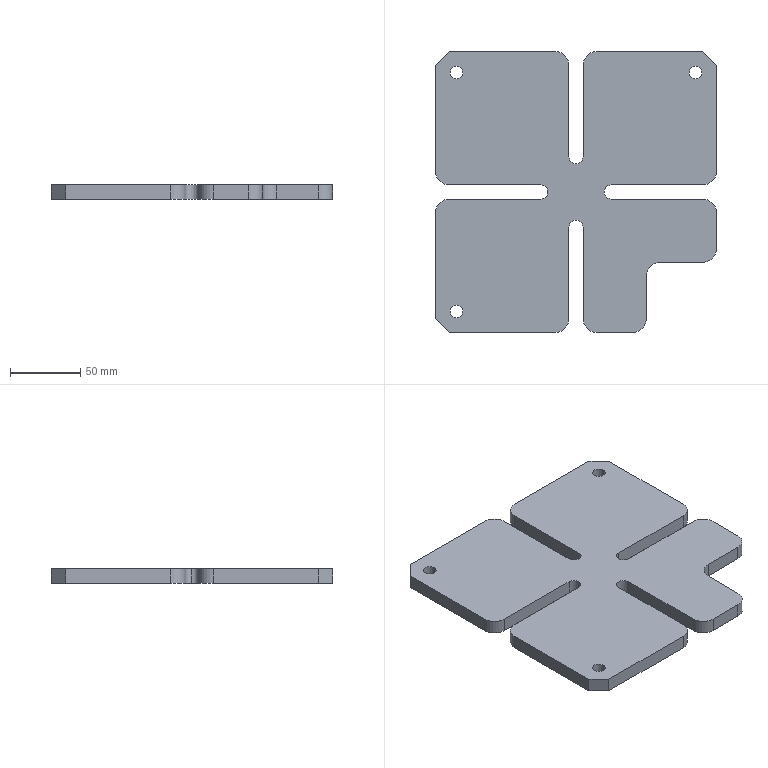Part | SolidWorks | features ICE 3, CirPattern 2, Fillet 2, Chamfer 1, DelFace 1, Extrusion 1, HoleWzd 1 | 1 solid | 45 faces | box 200 x 200 x 10 mm | volume 338089 mm3 | plane 23 | cylinder 22 | commonest cylinder face diameters 20 x11 9 x6 10 x5
STEP:
#1=CARTESIAN_POINT('',(-20.,0.,0.));
#2=VERTEX_POINT('',#1);
#3=CARTESIAN_POINT('',(-25.,5.,0.));
#4=VERTEX_POINT('',#3);
#5=CARTESIAN_POINT('',(-25.,0.,0.));
#6=DIRECTION('',(0.,0.,1.));
#7=DIRECTION('',(1.,0.,0.));
#8=AXIS2_PLACEMENT_3D('',#5,#6,#7);
#9=CIRCLE('',#8,5.);
#10=EDGE_CURVE('',#2,#4,#9,.T.);
#11=ORIENTED_EDGE('',*,*,#10,.F.);
#12=CARTESIAN_POINT('',(-20.,0.,10.));
#13=VERTEX_POINT('',#12);
#14=CARTESIAN_POINT('',(-20.,0.,-18.));
#15=DIRECTION('',(0.,0.,1.));
#16=VECTOR('',#15,1000.);
#17=LINE('',#14,#16);
#18=EDGE_CURVE('',#2,#13,#17,.T.);
#19=ORIENTED_EDGE('',*,*,#18,.T.);
#20=CARTESIAN_POINT('',(-25.,5.,10.));
#21=VERTEX_POINT('',#20);
#22=CARTESIAN_POINT('',(-25.,0.,10.));
#23=DIRECTION('',(0.,0.,1.));
#24=DIRECTION('',(1.,0.,0.));
#25=AXIS2_PLACEMENT_3D('',#22,#23,#24);
#26=CIRCLE('',#25,5.);
#27=EDGE_CURVE('',#13,#21,#26,.T.);
#28=ORIENTED_EDGE('',*,*,#27,.T.);
#29=CARTESIAN_POINT('',(-25.,5.,-18.));
#30=DIRECTION('',(0.,0.,1.));
#31=VECTOR('',#30,1000.);
#32=LINE('',#29,#31);
#33=EDGE_CURVE('',#4,#21,#32,.T.);
#34=ORIENTED_EDGE('',*,*,#33,.F.);
#35=EDGE_LOOP('',(#11,#19,#28,#34));
#36=FACE_OUTER_BOUND('',#35,.T.);
#37=CARTESIAN_POINT('',(-25.,0.,-18.));
#38=DIRECTION('',(0.,0.,1.));
#39=DIRECTION('',(1.,0.,0.));
#40=AXIS2_PLACEMENT_3D('',#37,#38,#39);
#41=CYLINDRICAL_SURFACE('',#40,5.);
#42=ADVANCED_FACE('',(#36),#41,.F.);
#43=CARTESIAN_POINT('',(80.5,85.,0.));
#44=VERTEX_POINT('',#43);
#45=CARTESIAN_POINT('',(89.5,85.,0.));
#46=VERTEX_POINT('',#45);
#47=CARTESIAN_POINT('',(85.,85.,0.));
#48=DIRECTION('',(0.,0.,1.));
#49=DIRECTION('',(1.,0.,0.));
#50=AXIS2_PLACEMENT_3D('',#47,#48,#49);
#51=CIRCLE('',#50,4.5);
#52=EDGE_CURVE('',#44,#46,#51,.T.);
#53=ORIENTED_EDGE('',*,*,#52,.F.);
#54=CARTESIAN_POINT('',(80.5,85.,10.));
#55=VERTEX_POINT('',#54);
#56=CARTESIAN_POINT('',(80.5,85.,10.));
#57=DIRECTION('',(0.,0.,1.));
#58=VECTOR('',#57,1000.);
#59=LINE('',#56,#58);
#60=EDGE_CURVE('',#44,#55,#59,.T.);
#61=ORIENTED_EDGE('',*,*,#60,.T.);
#62=CARTESIAN_POINT('',(89.5,85.,10.));
#63=VERTEX_POINT('',#62);
#64=CARTESIAN_POINT('',(85.,85.,10.));
#65=DIRECTION('',(0.,0.,1.));
#66=DIRECTION('',(1.,0.,0.));
#67=AXIS2_PLACEMENT_3D('',#64,#65,#66);
#68=CIRCLE('',#67,4.5);
#69=EDGE_CURVE('',#55,#63,#68,.T.);
#70=ORIENTED_EDGE('',*,*,#69,.T.);
#71=CARTESIAN_POINT('',(89.5,85.,10.));
#72=DIRECTION('',(0.,0.,1.));
#73=VECTOR('',#72,1000.);
#74=LINE('',#71,#73);
#75=EDGE_CURVE('',#46,#63,#74,.T.);
#76=ORIENTED_EDGE('',*,*,#75,.F.);
#77=EDGE_LOOP('',(#53,#61,#70,#76));
#78=FACE_OUTER_BOUND('',#77,.T.);
#79=CARTESIAN_POINT('',(85.,85.,10.));
#80=DIRECTION('',(0.,0.,1.));
#81=DIRECTION('',(1.,0.,0.));
#82=AXIS2_PLACEMENT_3D('',#79,#80,#81);
#83=CYLINDRICAL_SURFACE('',#82,4.5);
#84=ADVANCED_FACE('',(#78),#83,.F.);
#85=CARTESIAN_POINT('',(-89.5,85.,0.));
#86=VERTEX_POINT('',#85);
#87=CARTESIAN_POINT('',(-80.5,85.,0.));
#88=VERTEX_POINT('',#87);
#89=CARTESIAN_POINT('',(-85.,85.,0.));
#90=DIRECTION('',(0.,0.,1.));
#91=DIRECTION('',(1.,0.,0.));
#92=AXIS2_PLACEMENT_3D('',#89,#90,#91);
#93=CIRCLE('',#92,4.5);
#94=EDGE_CURVE('',#86,#88,#93,.T.);
#95=ORIENTED_EDGE('',*,*,#94,.F.);
#96=CARTESIAN_POINT('',(-89.5,85.,10.));
#97=VERTEX_POINT('',#96);
#98=CARTESIAN_POINT('',(-89.5,85.,10.));
#99=DIRECTION('',(0.,0.,1.));
#100=VECTOR('',#99,1000.);
#101=LINE('',#98,#100);
#102=EDGE_CURVE('',#86,#97,#101,.T.);
#103=ORIENTED_EDGE('',*,*,#102,.T.);
#104=CARTESIAN_POINT('',(-80.5,85.,10.));
#105=VERTEX_POINT('',#104);
#106=CARTESIAN_POINT('',(-85.,85.,10.));
#107=DIRECTION('',(0.,0.,1.));
#108=DIRECTION('',(1.,0.,0.));
#109=AXIS2_PLACEMENT_3D('',#106,#107,#108);
#110=CIRCLE('',#109,4.5);
#111=EDGE_CURVE('',#97,#105,#110,.T.);
#112=ORIENTED_EDGE('',*,*,#111,.T.);
#113=CARTESIAN_POINT('',(-80.5,85.,10.));
#114=DIRECTION('',(0.,0.,1.));
#115=VECTOR('',#114,1000.);
#116=LINE('',#113,#115);
#117=EDGE_CURVE('',#88,#105,#116,.T.);
#118=ORIENTED_EDGE('',*,*,#117,.F.);
#119=EDGE_LOOP('',(#95,#103,#112,#118));
#120=FACE_OUTER_BOUND('',#119,.T.);
#121=CARTESIAN_POINT('',(-85.,85.,10.));
#122=DIRECTION('',(0.,0.,1.));
#123=DIRECTION('',(1.,0.,0.));
#124=AXIS2_PLACEMENT_3D('',#121,#122,#123);
#125=CYLINDRICAL_SURFACE('',#124,4.5);
#126=ADVANCED_FACE('',(#120),#125,.F.);
#127=CARTESIAN_POINT('',(-89.5,-85.,0.));
#128=VERTEX_POINT('',#127);
#129=CARTESIAN_POINT('',(-80.5,-85.,0.));
#130=VERTEX_POINT('',#129);
#131=CARTESIAN_POINT('',(-85.,-85.,0.));
#132=DIRECTION('',(0.,0.,1.));
#133=DIRECTION('',(1.,0.,0.));
#134=AXIS2_PLACEMENT_3D('',#131,#132,#133);
#135=CIRCLE('',#134,4.5);
#136=EDGE_CURVE('',#128,#130,#135,.T.);
#137=ORIENTED_EDGE('',*,*,#136,.F.);
#138=CARTESIAN_POINT('',(-89.5,-85.,10.));
#139=VERTEX_POINT('',#138);
#140=CARTESIAN_POINT('',(-89.5,-85.,10.));
#141=DIRECTION('',(0.,0.,1.));
#142=VECTOR('',#141,1000.);
#143=LINE('',#140,#142);
#144=EDGE_CURVE('',#128,#139,#143,.T.);
#145=ORIENTED_EDGE('',*,*,#144,.T.);
#146=CARTESIAN_POINT('',(-80.5,-85.,10.));
#147=VERTEX_POINT('',#146);
#148=CARTESIAN_POINT('',(-85.,-85.,10.));
#149=DIRECTION('',(0.,0.,1.));
#150=DIRECTION('',(1.,0.,0.));
#151=AXIS2_PLACEMENT_3D('',#148,#149,#150);
#152=CIRCLE('',#151,4.5);
#153=EDGE_CURVE('',#139,#147,#152,.T.);
#154=ORIENTED_EDGE('',*,*,#153,.T.);
#155=CARTESIAN_POINT('',(-80.5,-85.,10.));
#156=DIRECTION('',(0.,0.,1.));
#157=VECTOR('',#156,1000.);
#158=LINE('',#155,#157);
#159=EDGE_CURVE('',#130,#147,#158,.T.);
#160=ORIENTED_EDGE('',*,*,#159,.F.);
#161=EDGE_LOOP('',(#137,#145,#154,#160));
#162=FACE_OUTER_BOUND('',#161,.T.);
#163=CARTESIAN_POINT('',(-85.,-85.,10.));
#164=DIRECTION('',(0.,0.,1.));
#165=DIRECTION('',(1.,0.,0.));
#166=AXIS2_PLACEMENT_3D('',#163,#164,#165);
#167=CYLINDRICAL_SURFACE('',#166,4.5);
#168=ADVANCED_FACE('',(#162),#167,.F.);
#169=CARTESIAN_POINT('',(100.,15.,10.));
#170=VERTEX_POINT('',#169);
#171=CARTESIAN_POINT('',(100.,90.,10.));
#172=VERTEX_POINT('',#171);
#173=CARTESIAN_POINT('',(100.,100.,10.));
#174=DIRECTION('',(0.,1.,0.));
#175=VECTOR('',#174,1000.);
#176=LINE('',#173,#175);
#177=EDGE_CURVE('',#170,#172,#176,.T.);
#178=ORIENTED_EDGE('',*,*,#177,.F.);
#179=CARTESIAN_POINT('',(100.,15.,0.));
#180=VERTEX_POINT('',#179);
#181=CARTESIAN_POINT('',(100.,15.,10.));
#182=DIRECTION('',(0.,0.,-1.));
#183=VECTOR('',#182,1000.);
#184=LINE('',#181,#183);
#185=EDGE_CURVE('',#170,#180,#184,.T.);
#186=ORIENTED_EDGE('',*,*,#185,.T.);
#187=CARTESIAN_POINT('',(100.,90.,0.));
#188=VERTEX_POINT('',#187);
#189=CARTESIAN_POINT('',(100.,100.,0.));
#190=DIRECTION('',(0.,1.,0.));
#191=VECTOR('',#190,1000.);
#192=LINE('',#189,#191);
#193=EDGE_CURVE('',#180,#188,#192,.T.);
#194=ORIENTED_EDGE('',*,*,#193,.T.);
#195=CARTESIAN_POINT('',(100.,90.,10.));
#196=DIRECTION('',(0.,0.,1.));
#197=VECTOR('',#196,1000.);
#198=LINE('',#195,#197);
#199=EDGE_CURVE('',#188,#172,#198,.T.);
#200=ORIENTED_EDGE('',*,*,#199,.T.);
#201=EDGE_LOOP('',(#178,#186,#194,#200));
#202=FACE_OUTER_BOUND('',#201,.T.);
#203=CARTESIAN_POINT('',(100.,100.,10.));
#204=DIRECTION('',(-1.,0.,0.));
#205=DIRECTION('',(0.,-1.,0.));
#206=AXIS2_PLACEMENT_3D('',#203,#204,#205);
#207=PLANE('',#206);
#208=ADVANCED_FACE('',(#202),#207,.F.);
#209=CARTESIAN_POINT('',(-15.,100.,10.));
#210=VERTEX_POINT('',#209);
#211=CARTESIAN_POINT('',(-90.,100.,10.));
#212=VERTEX_POINT('',#211);
#213=CARTESIAN_POINT('',(-100.,100.,10.));
#214=DIRECTION('',(-1.,0.,0.));
#215=VECTOR('',#214,1000.);
#216=LINE('',#213,#215);
#217=EDGE_CURVE('',#210,#212,#216,.T.);
#218=ORIENTED_EDGE('',*,*,#217,.F.);
#219=CARTESIAN_POINT('',(-15.,100.,0.));
#220=VERTEX_POINT('',#219);
#221=CARTESIAN_POINT('',(-15.,100.,10.));
#222=DIRECTION('',(0.,0.,-1.));
#223=VECTOR('',#222,1000.);
#224=LINE('',#221,#223);
#225=EDGE_CURVE('',#210,#220,#224,.T.);
#226=ORIENTED_EDGE('',*,*,#225,.T.);
#227=CARTESIAN_POINT('',(-90.,100.,0.));
#228=VERTEX_POINT('',#227);
#229=CARTESIAN_POINT('',(-100.,100.,0.));
#230=DIRECTION('',(-1.,0.,0.));
#231=VECTOR('',#230,1000.);
#232=LINE('',#229,#231);
#233=EDGE_CURVE('',#220,#228,#232,.T.);
#234=ORIENTED_EDGE('',*,*,#233,.T.);
#235=CARTESIAN_POINT('',(-90.,100.,10.));
#236=DIRECTION('',(0.,0.,1.));
#237=VECTOR('',#236,1000.);
#238=LINE('',#235,#237);
#239=EDGE_CURVE('',#228,#212,#238,.T.);
#240=ORIENTED_EDGE('',*,*,#239,.T.);
#241=EDGE_LOOP('',(#218,#226,#234,#240));
#242=FACE_OUTER_BOUND('',#241,.T.);
#243=CARTESIAN_POINT('',(-100.,100.,10.));
#244=DIRECTION('',(0.,-1.,0.));
#245=DIRECTION('',(0.,0.,-1.));
#246=AXIS2_PLACEMENT_3D('',#243,#244,#245);
#247=PLANE('',#246);
#248=ADVANCED_FACE('',(#242),#247,.F.);
#249=CARTESIAN_POINT('',(15.,-100.,0.));
#250=VERTEX_POINT('',#249);
#251=CARTESIAN_POINT('',(40.,-100.,0.));
#252=VERTEX_POINT('',#251);
#253=CARTESIAN_POINT('',(-100.,-100.,0.));
#254=DIRECTION('',(1.,0.,0.));
#255=VECTOR('',#254,1000.);
#256=LINE('',#253,#255);
#257=EDGE_CURVE('',#250,#252,#256,.T.);
#258=ORIENTED_EDGE('',*,*,#257,.T.);
#259=CARTESIAN_POINT('',(40.,-100.,10.));
#260=VERTEX_POINT('',#259);
#261=CARTESIAN_POINT('',(40.,-100.,10.));
#262=DIRECTION('',(0.,0.,1.));
#263=VECTOR('',#262,1000.);
#264=LINE('',#261,#263);
#265=EDGE_CURVE('',#252,#260,#264,.T.);
#266=ORIENTED_EDGE('',*,*,#265,.T.);
#267=CARTESIAN_POINT('',(15.,-100.,10.));
#268=VERTEX_POINT('',#267);
#269=CARTESIAN_POINT('',(-100.,-100.,10.));
#270=DIRECTION('',(1.,0.,0.));
#271=VECTOR('',#270,1000.);
#272=LINE('',#269,#271);
#273=EDGE_CURVE('',#268,#260,#272,.T.);
#274=ORIENTED_EDGE('',*,*,#273,.F.);
#275=CARTESIAN_POINT('',(15.,-100.,10.));
#276=DIRECTION('',(0.,0.,-1.));
#277=VECTOR('',#276,1000.);
#278=LINE('',#275,#277);
#279=EDGE_CURVE('',#268,#250,#278,.T.);
#280=ORIENTED_EDGE('',*,*,#279,.T.);
#281=EDGE_LOOP('',(#258,#266,#274,#280));
#282=FACE_OUTER_BOUND('',#281,.T.);
#283=CARTESIAN_POINT('',(-100.,-100.,10.));
#284=DIRECTION('',(0.,1.,0.));
#285=DIRECTION('',(0.,0.,1.));
#286=AXIS2_PLACEMENT_3D('',#283,#284,#285);
#287=PLANE('',#286);
#288=ADVANCED_FACE('',(#282),#287,.F.);
#289=CARTESIAN_POINT('',(-100.,-15.,10.));
#290=VERTEX_POINT('',#289);
#291=CARTESIAN_POINT('',(-100.,-90.,10.));
#292=VERTEX_POINT('',#291);
#293=CARTESIAN_POINT('',(-100.,100.,10.));
#294=DIRECTION('',(0.,-1.,0.));
#295=VECTOR('',#294,1000.);
#296=LINE('',#293,#295);
#297=EDGE_CURVE('',#290,#292,#296,.T.);
#298=ORIENTED_EDGE('',*,*,#297,.F.);
#299=CARTESIAN_POINT('',(-100.,-15.,0.));
#300=VERTEX_POINT('',#299);
#301=CARTESIAN_POINT('',(-100.,-15.,10.));
#302=DIRECTION('',(0.,0.,-1.));
#303=VECTOR('',#302,1000.);
#304=LINE('',#301,#303);
#305=EDGE_CURVE('',#290,#300,#304,.T.);
#306=ORIENTED_EDGE('',*,*,#305,.T.);
#307=CARTESIAN_POINT('',(-100.,-90.,0.));
#308=VERTEX_POINT('',#307);
#309=CARTESIAN_POINT('',(-100.,100.,0.));
#310=DIRECTION('',(0.,-1.,0.));
#311=VECTOR('',#310,1000.);
#312=LINE('',#309,#311);
#313=EDGE_CURVE('',#300,#308,#312,.T.);
#314=ORIENTED_EDGE('',*,*,#313,.T.);
#315=CARTESIAN_POINT('',(-100.,-90.,10.));
#316=DIRECTION('',(0.,0.,1.));
#317=VECTOR('',#316,1000.);
#318=LINE('',#315,#317);
#319=EDGE_CURVE('',#308,#292,#318,.T.);
#320=ORIENTED_EDGE('',*,*,#319,.T.);
#321=EDGE_LOOP('',(#298,#306,#314,#320));
#322=FACE_OUTER_BOUND('',#321,.T.);
#323=CARTESIAN_POINT('',(-100.,100.,10.));
#324=DIRECTION('',(1.,0.,0.));
#325=DIRECTION('',(0.,1.,0.));
#326=AXIS2_PLACEMENT_3D('',#323,#324,#325);
#327=PLANE('',#326);
#328=ADVANCED_FACE('',(#322),#327,.F.);
#329=CARTESIAN_POINT('',(100.,-40.,10.));
#330=VERTEX_POINT('',#329);
#331=CARTESIAN_POINT('',(100.,-15.,10.));
#332=VERTEX_POINT('',#331);
#333=CARTESIAN_POINT('',(100.,100.,10.));
#334=DIRECTION('',(0.,1.,0.));
#335=VECTOR('',#334,1000.);
#336=LINE('',#333,#335);
#337=EDGE_CURVE('',#330,#332,#336,.T.);
#338=ORIENTED_EDGE('',*,*,#337,.F.);
#339=CARTESIAN_POINT('',(100.,-40.,0.));
#340=VERTEX_POINT('',#339);
#341=CARTESIAN_POINT('',(100.,-40.,10.));
#342=DIRECTION('',(0.,0.,-1.));
#343=VECTOR('',#342,1000.);
#344=LINE('',#341,#343);
#345=EDGE_CURVE('',#330,#340,#344,.T.);
#346=ORIENTED_EDGE('',*,*,#345,.T.);
#347=CARTESIAN_POINT('',(100.,-15.,0.));
#348=VERTEX_POINT('',#347);
#349=CARTESIAN_POINT('',(100.,100.,0.));
#350=DIRECTION('',(0.,1.,0.));
#351=VECTOR('',#350,1000.);
#352=LINE('',#349,#351);
#353=EDGE_CURVE('',#340,#348,#352,.T.);
#354=ORIENTED_EDGE('',*,*,#353,.T.);
#355=CARTESIAN_POINT('',(100.,-15.,10.));
#356=DIRECTION('',(0.,0.,1.));
#357=VECTOR('',#356,1000.);
#358=LINE('',#355,#357);
#359=EDGE_CURVE('',#348,#332,#358,.T.);
#360=ORIENTED_EDGE('',*,*,#359,.T.);
#361=EDGE_LOOP('',(#338,#346,#354,#360));
#362=FACE_OUTER_BOUND('',#361,.T.);
#363=CARTESIAN_POINT('',(100.,100.,10.));
#364=DIRECTION('',(-1.,0.,0.));
#365=DIRECTION('',(0.,-1.,0.));
#366=AXIS2_PLACEMENT_3D('',#363,#364,#365);
#367=PLANE('',#366);
#368=ADVANCED_FACE('',(#362),#367,.F.);
#369=CARTESIAN_POINT('',(90.,100.,0.));
#370=VERTEX_POINT('',#369);
#371=CARTESIAN_POINT('',(15.,100.,0.));
#372=VERTEX_POINT('',#371);
#373=CARTESIAN_POINT('',(-100.,100.,0.));
#374=DIRECTION('',(-1.,0.,0.));
#375=VECTOR('',#374,1000.);
#376=LINE('',#373,#375);
#377=EDGE_CURVE('',#370,#372,#376,.T.);
#378=ORIENTED_EDGE('',*,*,#377,.T.);
#379=CARTESIAN_POINT('',(15.,100.,10.));
#380=VERTEX_POINT('',#379);
#381=CARTESIAN_POINT('',(15.,100.,10.));
#382=DIRECTION('',(0.,0.,1.));
#383=VECTOR('',#382,1000.);
#384=LINE('',#381,#383);
#385=EDGE_CURVE('',#372,#380,#384,.T.);
#386=ORIENTED_EDGE('',*,*,#385,.T.);
#387=CARTESIAN_POINT('',(90.,100.,10.));
#388=VERTEX_POINT('',#387);
#389=CARTESIAN_POINT('',(-100.,100.,10.));
#390=DIRECTION('',(-1.,0.,0.));
#391=VECTOR('',#390,1000.);
#392=LINE('',#389,#391);
#393=EDGE_CURVE('',#388,#380,#392,.T.);
#394=ORIENTED_EDGE('',*,*,#393,.F.);
#395=CARTESIAN_POINT('',(90.,100.,10.));
#396=DIRECTION('',(0.,0.,-1.));
#397=VECTOR('',#396,1000.);
#398=LINE('',#395,#397);
#399=EDGE_CURVE('',#388,#370,#398,.T.);
#400=ORIENTED_EDGE('',*,*,#399,.T.);
#401=EDGE_LOOP('',(#378,#386,#394,#400));
#402=FACE_OUTER_BOUND('',#401,.T.);
#403=CARTESIAN_POINT('',(-100.,100.,10.));
#404=DIRECTION('',(0.,-1.,0.));
#405=DIRECTION('',(0.,0.,-1.));
#406=AXIS2_PLACEMENT_3D('',#403,#404,#405);
#407=PLANE('',#406);
#408=ADVANCED_FACE('',(#402),#407,.F.);
#409=CARTESIAN_POINT('',(-100.,90.,0.));
#410=VERTEX_POINT('',#409);
#411=CARTESIAN_POINT('',(-100.,15.,0.));
#412=VERTEX_POINT('',#411);
#413=CARTESIAN_POINT('',(-100.,100.,0.));
#414=DIRECTION('',(0.,-1.,0.));
#415=VECTOR('',#414,1000.);
#416=LINE('',#413,#415);
#417=EDGE_CURVE('',#410,#412,#416,.T.);
#418=ORIENTED_EDGE('',*,*,#417,.T.);
#419=CARTESIAN_POINT('',(-100.,15.,10.));
#420=VERTEX_POINT('',#419);
#421=CARTESIAN_POINT('',(-100.,15.,10.));
#422=DIRECTION('',(0.,0.,1.));
#423=VECTOR('',#422,1000.);
#424=LINE('',#421,#423);
#425=EDGE_CURVE('',#412,#420,#424,.T.);
#426=ORIENTED_EDGE('',*,*,#425,.T.);
#427=CARTESIAN_POINT('',(-100.,90.,10.));
#428=VERTEX_POINT('',#427);
#429=CARTESIAN_POINT('',(-100.,100.,10.));
#430=DIRECTION('',(0.,-1.,0.));
#431=VECTOR('',#430,1000.);
#432=LINE('',#429,#431);
#433=EDGE_CURVE('',#428,#420,#432,.T.);
#434=ORIENTED_EDGE('',*,*,#433,.F.);
#435=CARTESIAN_POINT('',(-100.,90.,10.));
#436=DIRECTION('',(0.,0.,-1.));
#437=VECTOR('',#436,1000.);
#438=LINE('',#435,#437);
#439=EDGE_CURVE('',#428,#410,#438,.T.);
#440=ORIENTED_EDGE('',*,*,#439,.T.);
#441=EDGE_LOOP('',(#418,#426,#434,#440));
#442=FACE_OUTER_BOUND('',#441,.T.);
#443=CARTESIAN_POINT('',(-100.,100.,10.));
#444=DIRECTION('',(1.,0.,0.));
#445=DIRECTION('',(0.,1.,0.));
#446=AXIS2_PLACEMENT_3D('',#443,#444,#445);
#447=PLANE('',#446);
#448=ADVANCED_FACE('',(#442),#447,.F.);
#449=CARTESIAN_POINT('',(-90.,-100.,0.));
#450=VERTEX_POINT('',#449);
#451=CARTESIAN_POINT('',(-15.,-100.,0.));
#452=VERTEX_POINT('',#451);
#453=CARTESIAN_POINT('',(-100.,-100.,0.));
#454=DIRECTION('',(1.,0.,0.));
#455=VECTOR('',#454,1000.);
#456=LINE('',#453,#455);
#457=EDGE_CURVE('',#450,#452,#456,.T.);
#458=ORIENTED_EDGE('',*,*,#457,.T.);
#459=CARTESIAN_POINT('',(-15.,-100.,10.));
#460=VERTEX_POINT('',#459);
#461=CARTESIAN_POINT('',(-15.,-100.,10.));
#462=DIRECTION('',(0.,0.,1.));
#463=VECTOR('',#462,1000.);
#464=LINE('',#461,#463);
#465=EDGE_CURVE('',#452,#460,#464,.T.);
#466=ORIENTED_EDGE('',*,*,#465,.T.);
#467=CARTESIAN_POINT('',(-90.,-100.,10.));
#468=VERTEX_POINT('',#467);
#469=CARTESIAN_POINT('',(-100.,-100.,10.));
#470=DIRECTION('',(1.,0.,0.));
#471=VECTOR('',#470,1000.);
#472=LINE('',#469,#471);
#473=EDGE_CURVE('',#468,#460,#472,.T.);
#474=ORIENTED_EDGE('',*,*,#473,.F.);
#475=CARTESIAN_POINT('',(-90.,-100.,10.));
#476=DIRECTION('',(0.,0.,-1.));
#477=VECTOR('',#476,1000.);
#478=LINE('',#475,#477);
#479=EDGE_CURVE('',#468,#450,#478,.T.);
#480=ORIENTED_EDGE('',*,*,#479,.T.);
#481=EDGE_LOOP('',(#458,#466,#474,#480));
#482=FACE_OUTER_BOUND('',#481,.T.);
#483=CARTESIAN_POINT('',(-100.,-100.,10.));
#484=DIRECTION('',(0.,1.,0.));
#485=DIRECTION('',(0.,0.,1.));
#486=AXIS2_PLACEMENT_3D('',#483,#484,#485);
#487=PLANE('',#486);
#488=ADVANCED_FACE('',(#482),#487,.F.);
#489=ORIENTED_EDGE('',*,*,#273,.T.);
#490=CARTESIAN_POINT('',(50.,-90.,10.));
#491=VERTEX_POINT('',#490);
#492=CARTESIAN_POINT('',(40.,-90.,10.));
#493=DIRECTION('',(0.,0.,1.));
#494=DIRECTION('',(1.,0.,0.));
#495=AXIS2_PLACEMENT_3D('',#492,#493,#494);
#496=CIRCLE('',#495,10.);
#497=EDGE_CURVE('',#260,#491,#496,.T.);
#498=ORIENTED_EDGE('',*,*,#497,.T.);
#499=CARTESIAN_POINT('',(50.,-60.,10.));
#500=VERTEX_POINT('',#499);
#501=CARTESIAN_POINT('',(50.,-50.,10.));
#502=DIRECTION('',(0.,-1.,0.));
#503=VECTOR('',#502,1000.);
#504=LINE('',#501,#503);
#505=EDGE_CURVE('',#500,#491,#504,.T.);
#506=ORIENTED_EDGE('',*,*,#505,.F.);
#507=CARTESIAN_POINT('',(60.,-50.,10.));
#508=VERTEX_POINT('',#507);
#509=CARTESIAN_POINT('',(60.,-60.,10.));
#510=DIRECTION('',(0.,0.,-1.));
#511=DIRECTION('',(1.,0.,0.));
#512=AXIS2_PLACEMENT_3D('',#509,#510,#511);
#513=CIRCLE('',#512,10.);
#514=EDGE_CURVE('',#500,#508,#513,.T.);
#515=ORIENTED_EDGE('',*,*,#514,.T.);
#516=CARTESIAN_POINT('',(90.,-50.,10.));
#517=VERTEX_POINT('',#516);
#518=CARTESIAN_POINT('',(50.,-50.,10.));
#519=DIRECTION('',(-1.,0.,0.));
#520=VECTOR('',#519,1000.);
#521=LINE('',#518,#520);
#522=EDGE_CURVE('',#517,#508,#521,.T.);
#523=ORIENTED_EDGE('',*,*,#522,.F.);
#524=CARTESIAN_POINT('',(90.,-40.,10.));
#525=DIRECTION('',(0.,0.,1.));
#526=DIRECTION('',(1.,0.,0.));
#527=AXIS2_PLACEMENT_3D('',#524,#525,#526);
#528=CIRCLE('',#527,10.);
#529=EDGE_CURVE('',#517,#330,#528,.T.);
#530=ORIENTED_EDGE('',*,*,#529,.T.);
#531=ORIENTED_EDGE('',*,*,#337,.T.);
#532=CARTESIAN_POINT('',(90.,-5.,10.));
#533=VERTEX_POINT('',#532);
#534=CARTESIAN_POINT('',(90.,-15.,10.));
#535=DIRECTION('',(0.,0.,1.));
#536=DIRECTION('',(1.,0.,0.));
#537=AXIS2_PLACEMENT_3D('',#534,#535,#536);
#538=CIRCLE('',#537,10.);
#539=EDGE_CURVE('',#332,#533,#538,.T.);
#540=ORIENTED_EDGE('',*,*,#539,.T.);
#541=CARTESIAN_POINT('',(25.,-5.,10.));
#542=VERTEX_POINT('',#541);
#543=CARTESIAN_POINT('',(25.,-5.,10.));
#544=DIRECTION('',(1.,0.,0.));
#545=VECTOR('',#544,1000.);
#546=LINE('',#543,#545);
#547=EDGE_CURVE('',#542,#533,#546,.T.);
#548=ORIENTED_EDGE('',*,*,#547,.F.);
#549=CARTESIAN_POINT('',(25.,5.,10.));
#550=VERTEX_POINT('',#549);
#551=CARTESIAN_POINT('',(25.,0.,10.));
#552=DIRECTION('',(0.,0.,1.));
#553=DIRECTION('',(-1.,0.,0.));
#554=AXIS2_PLACEMENT_3D('',#551,#552,#553);
#555=CIRCLE('',#554,5.);
#556=EDGE_CURVE('',#550,#542,#555,.T.);
#557=ORIENTED_EDGE('',*,*,#556,.F.);
#558=CARTESIAN_POINT('',(90.,5.,10.));
#559=VERTEX_POINT('',#558);
#560=CARTESIAN_POINT('',(25.,5.,10.));
#561=DIRECTION('',(-1.,0.,0.));
#562=VECTOR('',#561,1000.);
#563=LINE('',#560,#562);
#564=EDGE_CURVE('',#559,#550,#563,.T.);
#565=ORIENTED_EDGE('',*,*,#564,.F.);
#566=CARTESIAN_POINT('',(90.,15.,10.));
#567=DIRECTION('',(0.,0.,1.));
#568=DIRECTION('',(1.,0.,0.));
#569=AXIS2_PLACEMENT_3D('',#566,#567,#568);
#570=CIRCLE('',#569,10.);
#571=EDGE_CURVE('',#559,#170,#570,.T.);
#572=ORIENTED_EDGE('',*,*,#571,.T.);
#573=ORIENTED_EDGE('',*,*,#177,.T.);
#574=CARTESIAN_POINT('',(95.,95.,10.));
#575=DIRECTION('',(-0.7071,0.7071,0.));
#576=VECTOR('',#575,1000.);
#577=LINE('',#574,#576);
#578=EDGE_CURVE('',#172,#388,#577,.T.);
#579=ORIENTED_EDGE('',*,*,#578,.T.);
#580=ORIENTED_EDGE('',*,*,#393,.T.);
#581=CARTESIAN_POINT('',(5.,90.,10.));
#582=VERTEX_POINT('',#581);
#583=CARTESIAN_POINT('',(15.,90.,10.));
#584=DIRECTION('',(0.,0.,1.));
#585=DIRECTION('',(1.,0.,0.));
#586=AXIS2_PLACEMENT_3D('',#583,#584,#585);
#587=CIRCLE('',#586,10.);
#588=EDGE_CURVE('',#380,#582,#587,.T.);
#589=ORIENTED_EDGE('',*,*,#588,.T.);
#590=CARTESIAN_POINT('',(5.,25.,10.));
#591=VERTEX_POINT('',#590);
#592=CARTESIAN_POINT('',(5.,25.,10.));
#593=DIRECTION('',(0.,1.,0.));
#594=VECTOR('',#593,1000.);
#595=LINE('',#592,#594);
#596=EDGE_CURVE('',#591,#582,#595,.T.);
#597=ORIENTED_EDGE('',*,*,#596,.F.);
#598=CARTESIAN_POINT('',(-5.,25.,10.));
#599=VERTEX_POINT('',#598);
#600=CARTESIAN_POINT('',(0.,25.,10.));
#601=DIRECTION('',(0.,0.,1.));
#602=DIRECTION('',(0.,-1.,0.));
#603=AXIS2_PLACEMENT_3D('',#600,#601,#602);
#604=CIRCLE('',#603,5.);
#605=EDGE_CURVE('',#599,#591,#604,.T.);
#606=ORIENTED_EDGE('',*,*,#605,.F.);
#607=CARTESIAN_POINT('',(-5.,90.,10.));
#608=VERTEX_POINT('',#607);
#609=CARTESIAN_POINT('',(-5.,25.,10.));
#610=DIRECTION('',(0.,-1.,0.));
#611=VECTOR('',#610,1000.);
#612=LINE('',#609,#611);
#613=EDGE_CURVE('',#608,#599,#612,.T.);
#614=ORIENTED_EDGE('',*,*,#613,.F.);
#615=CARTESIAN_POINT('',(-15.,90.,10.));
#616=DIRECTION('',(0.,0.,1.));
#617=DIRECTION('',(1.,0.,0.));
#618=AXIS2_PLACEMENT_3D('',#615,#616,#617);
#619=CIRCLE('',#618,10.);
#620=EDGE_CURVE('',#608,#210,#619,.T.);
#621=ORIENTED_EDGE('',*,*,#620,.T.);
#622=ORIENTED_EDGE('',*,*,#217,.T.);
#623=CARTESIAN_POINT('',(-95.,95.,10.));
#624=DIRECTION('',(-0.7071,-0.7071,0.));
#625=VECTOR('',#624,1000.);
#626=LINE('',#623,#625);
#627=EDGE_CURVE('',#212,#428,#626,.T.);
#628=ORIENTED_EDGE('',*,*,#627,.T.);
#629=ORIENTED_EDGE('',*,*,#433,.T.);
#630=CARTESIAN_POINT('',(-90.,5.,10.));
#631=VERTEX_POINT('',#630);
#632=CARTESIAN_POINT('',(-90.,15.,10.));
#633=DIRECTION('',(0.,0.,1.));
#634=DIRECTION('',(1.,0.,0.));
#635=AXIS2_PLACEMENT_3D('',#632,#633,#634);
#636=CIRCLE('',#635,10.);
#637=EDGE_CURVE('',#420,#631,#636,.T.);
#638=ORIENTED_EDGE('',*,*,#637,.T.);
#639=CARTESIAN_POINT('',(-25.,5.,10.));
#640=DIRECTION('',(-1.,0.,0.));
#641=VECTOR('',#640,1000.);
#642=LINE('',#639,#641);
#643=EDGE_CURVE('',#21,#631,#642,.T.);
#644=ORIENTED_EDGE('',*,*,#643,.F.);
#645=ORIENTED_EDGE('',*,*,#27,.F.);
#646=CARTESIAN_POINT('',(-25.,-5.,10.));
#647=VERTEX_POINT('',#646);
#648=CARTESIAN_POINT('',(-25.,0.,10.));
#649=DIRECTION('',(0.,0.,1.));
#650=DIRECTION('',(1.,0.,0.));
#651=AXIS2_PLACEMENT_3D('',#648,#649,#650);
#652=CIRCLE('',#651,5.);
#653=EDGE_CURVE('',#647,#13,#652,.T.);
#654=ORIENTED_EDGE('',*,*,#653,.F.);
#655=CARTESIAN_POINT('',(-90.,-5.,10.));
#656=VERTEX_POINT('',#655);
#657=CARTESIAN_POINT('',(-25.,-5.,10.));
#658=DIRECTION('',(1.,0.,0.));
#659=VECTOR('',#658,1000.);
#660=LINE('',#657,#659);
#661=EDGE_CURVE('',#656,#647,#660,.T.);
#662=ORIENTED_EDGE('',*,*,#661,.F.);
#663=CARTESIAN_POINT('',(-90.,-15.,10.));
#664=DIRECTION('',(0.,0.,1.));
#665=DIRECTION('',(1.,0.,0.));
#666=AXIS2_PLACEMENT_3D('',#663,#664,#665);
#667=CIRCLE('',#666,10.);
#668=EDGE_CURVE('',#656,#290,#667,.T.);
#669=ORIENTED_EDGE('',*,*,#668,.T.);
#670=ORIENTED_EDGE('',*,*,#297,.T.);
#671=CARTESIAN_POINT('',(-95.,-95.,10.));
#672=DIRECTION('',(0.7071,-0.7071,0.));
#673=VECTOR('',#672,1000.);
#674=LINE('',#671,#673);
#675=EDGE_CURVE('',#292,#468,#674,.T.);
#676=ORIENTED_EDGE('',*,*,#675,.T.);
#677=ORIENTED_EDGE('',*,*,#473,.T.);
#678=CARTESIAN_POINT('',(-5.,-90.,10.));
#679=VERTEX_POINT('',#678);
#680=CARTESIAN_POINT('',(-15.,-90.,10.));
#681=DIRECTION('',(0.,0.,1.));
#682=DIRECTION('',(1.,0.,0.));
#683=AXIS2_PLACEMENT_3D('',#680,#681,#682);
#684=CIRCLE('',#683,10.);
#685=EDGE_CURVE('',#460,#679,#684,.T.);
#686=ORIENTED_EDGE('',*,*,#685,.T.);
#687=CARTESIAN_POINT('',(-5.,-25.,10.));
#688=VERTEX_POINT('',#687);
#689=CARTESIAN_POINT('',(-5.,-25.,10.));
#690=DIRECTION('',(0.,-1.,0.));
#691=VECTOR('',#690,1000.);
#692=LINE('',#689,#691);
#693=EDGE_CURVE('',#688,#679,#692,.T.);
#694=ORIENTED_EDGE('',*,*,#693,.F.);
#695=CARTESIAN_POINT('',(5.,-25.,10.));
#696=VERTEX_POINT('',#695);
#697=CARTESIAN_POINT('',(0.,-25.,10.));
#698=DIRECTION('',(0.,0.,1.));
#699=DIRECTION('',(0.,1.,0.));
#700=AXIS2_PLACEMENT_3D('',#697,#698,#699);
#701=CIRCLE('',#700,5.);
#702=EDGE_CURVE('',#696,#688,#701,.T.);
#703=ORIENTED_EDGE('',*,*,#702,.F.);
#704=CARTESIAN_POINT('',(5.,-90.,10.));
#705=VERTEX_POINT('',#704);
#706=CARTESIAN_POINT('',(5.,-25.,10.));
#707=DIRECTION('',(0.,1.,0.));
#708=VECTOR('',#707,1000.);
#709=LINE('',#706,#708);
#710=EDGE_CURVE('',#705,#696,#709,.T.);
#711=ORIENTED_EDGE('',*,*,#710,.F.);
#712=CARTESIAN_POINT('',(15.,-90.,10.));
#713=DIRECTION('',(0.,0.,1.));
#714=DIRECTION('',(1.,0.,0.));
#715=AXIS2_PLACEMENT_3D('',#712,#713,#714);
#716=CIRCLE('',#715,10.);
#717=EDGE_CURVE('',#705,#268,#716,.T.);
#718=ORIENTED_EDGE('',*,*,#717,.T.);
#719=EDGE_LOOP('',(#489,#498,#506,#515,#523,#530,#531,#540,#548,#557,#565,#572,#573,#579,#580,#589,#597,#606,#614,#621,#622,#628,#629,#638,#644,#645,#654,#662,#669,#670,#676,#677,#686,#694,#703,#711,#718));
#720=FACE_OUTER_BOUND('',#719,.T.);
#721=CARTESIAN_POINT('',(85.,85.,10.));
#722=DIRECTION('',(0.,0.,1.));
#723=DIRECTION('',(1.,0.,0.));
#724=AXIS2_PLACEMENT_3D('',#721,#722,#723);
#725=CIRCLE('',#724,4.5);
#726=EDGE_CURVE('',#63,#55,#725,.T.);
#727=ORIENTED_EDGE('',*,*,#726,.F.);
#728=ORIENTED_EDGE('',*,*,#69,.F.);
#729=EDGE_LOOP('',(#727,#728));
#730=FACE_BOUND('',#729,.T.);
#731=CARTESIAN_POINT('',(-85.,85.,10.));
#732=DIRECTION('',(0.,0.,1.));
#733=DIRECTION('',(1.,0.,0.));
#734=AXIS2_PLACEMENT_3D('',#731,#732,#733);
#735=CIRCLE('',#734,4.5);
#736=EDGE_CURVE('',#105,#97,#735,.T.);
#737=ORIENTED_EDGE('',*,*,#736,.F.);
#738=ORIENTED_EDGE('',*,*,#111,.F.);
#739=EDGE_LOOP('',(#737,#738));
#740=FACE_BOUND('',#739,.T.);
#741=CARTESIAN_POINT('',(-85.,-85.,10.));
#742=DIRECTION('',(0.,0.,1.));
#743=DIRECTION('',(1.,0.,0.));
#744=AXIS2_PLACEMENT_3D('',#741,#742,#743);
#745=CIRCLE('',#744,4.5);
#746=EDGE_CURVE('',#147,#139,#745,.T.);
#747=ORIENTED_EDGE('',*,*,#746,.F.);
#748=ORIENTED_EDGE('',*,*,#153,.F.);
#749=EDGE_LOOP('',(#747,#748));
#750=FACE_BOUND('',#749,.T.);
#751=CARTESIAN_POINT('',(0.,0.,10.));
#752=DIRECTION('',(0.,0.,1.));
#753=DIRECTION('',(1.,0.,0.));
#754=AXIS2_PLACEMENT_3D('',#751,#752,#753);
#755=PLANE('',#754);
#756=ADVANCED_FACE('',(#720,#730,#740,#750),#755,.T.);
#757=CARTESIAN_POINT('',(85.,85.,0.));
#758=DIRECTION('',(0.,0.,1.));
#759=DIRECTION('',(1.,0.,0.));
#760=AXIS2_PLACEMENT_3D('',#757,#758,#759);
#761=CIRCLE('',#760,4.5);
#762=EDGE_CURVE('',#46,#44,#761,.T.);
#763=ORIENTED_EDGE('',*,*,#762,.T.);
#764=ORIENTED_EDGE('',*,*,#52,.T.);
#765=EDGE_LOOP('',(#763,#764));
#766=FACE_BOUND('',#765,.T.);
#767=CARTESIAN_POINT('',(-85.,85.,0.));
#768=DIRECTION('',(0.,0.,1.));
#769=DIRECTION('',(1.,0.,0.));
#770=AXIS2_PLACEMENT_3D('',#767,#768,#769);
#771=CIRCLE('',#770,4.5);
#772=EDGE_CURVE('',#88,#86,#771,.T.);
#773=ORIENTED_EDGE('',*,*,#772,.T.);
#774=ORIENTED_EDGE('',*,*,#94,.T.);
#775=EDGE_LOOP('',(#773,#774));
#776=FACE_BOUND('',#775,.T.);
#777=CARTESIAN_POINT('',(-85.,-85.,0.));
#778=DIRECTION('',(0.,0.,1.));
#779=DIRECTION('',(1.,0.,0.));
#780=AXIS2_PLACEMENT_3D('',#777,#778,#779);
#781=CIRCLE('',#780,4.5);
#782=EDGE_CURVE('',#130,#128,#781,.T.);
#783=ORIENTED_EDGE('',*,*,#782,.T.);
#784=ORIENTED_EDGE('',*,*,#136,.T.);
#785=EDGE_LOOP('',(#783,#784));
#786=FACE_BOUND('',#785,.T.);
#787=CARTESIAN_POINT('',(50.,-60.,0.));
#788=VERTEX_POINT('',#787);
#789=CARTESIAN_POINT('',(50.,-90.,0.));
#790=VERTEX_POINT('',#789);
#791=CARTESIAN_POINT('',(50.,-50.,0.));
#792=DIRECTION('',(0.,-1.,0.));
#793=VECTOR('',#792,1000.);
#794=LINE('',#791,#793);
#795=EDGE_CURVE('',#788,#790,#794,.T.);
#796=ORIENTED_EDGE('',*,*,#795,.T.);
#797=CARTESIAN_POINT('',(40.,-90.,0.));
#798=DIRECTION('',(0.,0.,-1.));
#799=DIRECTION('',(1.,0.,0.));
#800=AXIS2_PLACEMENT_3D('',#797,#798,#799);
#801=CIRCLE('',#800,10.);
#802=EDGE_CURVE('',#790,#252,#801,.T.);
#803=ORIENTED_EDGE('',*,*,#802,.T.);
#804=ORIENTED_EDGE('',*,*,#257,.F.);
#805=CARTESIAN_POINT('',(5.,-90.,0.));
#806=VERTEX_POINT('',#805);
#807=CARTESIAN_POINT('',(15.,-90.,0.));
#808=DIRECTION('',(0.,0.,-1.));
#809=DIRECTION('',(1.,0.,0.));
#810=AXIS2_PLACEMENT_3D('',#807,#808,#809);
#811=CIRCLE('',#810,10.);
#812=EDGE_CURVE('',#250,#806,#811,.T.);
#813=ORIENTED_EDGE('',*,*,#812,.T.);
#814=CARTESIAN_POINT('',(5.,-25.,0.));
#815=VERTEX_POINT('',#814);
#816=CARTESIAN_POINT('',(5.,0.,0.));
#817=DIRECTION('',(0.,1.,0.));
#818=VECTOR('',#817,1000.);
#819=LINE('',#816,#818);
#820=EDGE_CURVE('',#806,#815,#819,.T.);
#821=ORIENTED_EDGE('',*,*,#820,.T.);
#822=CARTESIAN_POINT('',(-5.,-25.,0.));
#823=VERTEX_POINT('',#822);
#824=CARTESIAN_POINT('',(0.,-25.,0.));
#825=DIRECTION('',(0.,0.,1.));
#826=DIRECTION('',(1.,0.,0.));
#827=AXIS2_PLACEMENT_3D('',#824,#825,#826);
#828=CIRCLE('',#827,5.);
#829=EDGE_CURVE('',#815,#823,#828,.T.);
#830=ORIENTED_EDGE('',*,*,#829,.T.);
#831=CARTESIAN_POINT('',(-5.,-90.,0.));
#832=VERTEX_POINT('',#831);
#833=CARTESIAN_POINT('',(-5.,0.,0.));
#834=DIRECTION('',(0.,-1.,0.));
#835=VECTOR('',#834,1000.);
#836=LINE('',#833,#835);
#837=EDGE_CURVE('',#823,#832,#836,.T.);
#838=ORIENTED_EDGE('',*,*,#837,.T.);
#839=CARTESIAN_POINT('',(-15.,-90.,0.));
#840=DIRECTION('',(0.,0.,-1.));
#841=DIRECTION('',(1.,0.,0.));
#842=AXIS2_PLACEMENT_3D('',#839,#840,#841);
#843=CIRCLE('',#842,10.);
#844=EDGE_CURVE('',#832,#452,#843,.T.);
#845=ORIENTED_EDGE('',*,*,#844,.T.);
#846=ORIENTED_EDGE('',*,*,#457,.F.);
#847=CARTESIAN_POINT('',(-90.,-100.,0.));
#848=DIRECTION('',(-0.7071,0.7071,0.));
#849=VECTOR('',#848,1000.);
#850=LINE('',#847,#849);
#851=EDGE_CURVE('',#450,#308,#850,.T.);
#852=ORIENTED_EDGE('',*,*,#851,.T.);
#853=ORIENTED_EDGE('',*,*,#313,.F.);
#854=CARTESIAN_POINT('',(-90.,-5.,0.));
#855=VERTEX_POINT('',#854);
#856=CARTESIAN_POINT('',(-90.,-15.,0.));
#857=DIRECTION('',(0.,0.,-1.));
#858=DIRECTION('',(1.,0.,0.));
#859=AXIS2_PLACEMENT_3D('',#856,#857,#858);
#860=CIRCLE('',#859,10.);
#861=EDGE_CURVE('',#300,#855,#860,.T.);
#862=ORIENTED_EDGE('',*,*,#861,.T.);
#863=CARTESIAN_POINT('',(-25.,-5.,0.));
#864=VERTEX_POINT('',#863);
#865=CARTESIAN_POINT('',(0.,-5.,0.));
#866=DIRECTION('',(1.,0.,0.));
#867=VECTOR('',#866,1000.);
#868=LINE('',#865,#867);
#869=EDGE_CURVE('',#855,#864,#868,.T.);
#870=ORIENTED_EDGE('',*,*,#869,.T.);
#871=CARTESIAN_POINT('',(-25.,0.,0.));
#872=DIRECTION('',(0.,0.,1.));
#873=DIRECTION('',(1.,0.,0.));
#874=AXIS2_PLACEMENT_3D('',#871,#872,#873);
#875=CIRCLE('',#874,5.);
#876=EDGE_CURVE('',#864,#2,#875,.T.);
#877=ORIENTED_EDGE('',*,*,#876,.T.);
#878=ORIENTED_EDGE('',*,*,#10,.T.);
#879=CARTESIAN_POINT('',(-90.,5.,0.));
#880=VERTEX_POINT('',#879);
#881=CARTESIAN_POINT('',(0.,5.,0.));
#882=DIRECTION('',(-1.,0.,0.));
#883=VECTOR('',#882,1000.);
#884=LINE('',#881,#883);
#885=EDGE_CURVE('',#4,#880,#884,.T.);
#886=ORIENTED_EDGE('',*,*,#885,.T.);
#887=CARTESIAN_POINT('',(-90.,15.,0.));
#888=DIRECTION('',(0.,0.,-1.));
#889=DIRECTION('',(1.,0.,0.));
#890=AXIS2_PLACEMENT_3D('',#887,#888,#889);
#891=CIRCLE('',#890,10.);
#892=EDGE_CURVE('',#880,#412,#891,.T.);
#893=ORIENTED_EDGE('',*,*,#892,.T.);
#894=ORIENTED_EDGE('',*,*,#417,.F.);
#895=CARTESIAN_POINT('',(-100.,90.,0.));
#896=DIRECTION('',(0.7071,0.7071,0.));
#897=VECTOR('',#896,1000.);
#898=LINE('',#895,#897);
#899=EDGE_CURVE('',#410,#228,#898,.T.);
#900=ORIENTED_EDGE('',*,*,#899,.T.);
#901=ORIENTED_EDGE('',*,*,#233,.F.);
#902=CARTESIAN_POINT('',(-5.,90.,0.));
#903=VERTEX_POINT('',#902);
#904=CARTESIAN_POINT('',(-15.,90.,0.));
#905=DIRECTION('',(0.,0.,-1.));
#906=DIRECTION('',(1.,0.,0.));
#907=AXIS2_PLACEMENT_3D('',#904,#905,#906);
#908=CIRCLE('',#907,10.);
#909=EDGE_CURVE('',#220,#903,#908,.T.);
#910=ORIENTED_EDGE('',*,*,#909,.T.);
#911=CARTESIAN_POINT('',(-5.,25.,0.));
#912=VERTEX_POINT('',#911);
#913=CARTESIAN_POINT('',(-5.,0.,0.));
#914=DIRECTION('',(0.,-1.,0.));
#915=VECTOR('',#914,1000.);
#916=LINE('',#913,#915);
#917=EDGE_CURVE('',#903,#912,#916,.T.);
#918=ORIENTED_EDGE('',*,*,#917,.T.);
#919=CARTESIAN_POINT('',(5.,25.,0.));
#920=VERTEX_POINT('',#919);
#921=CARTESIAN_POINT('',(0.,25.,0.));
#922=DIRECTION('',(0.,0.,1.));
#923=DIRECTION('',(1.,0.,0.));
#924=AXIS2_PLACEMENT_3D('',#921,#922,#923);
#925=CIRCLE('',#924,5.);
#926=EDGE_CURVE('',#912,#920,#925,.T.);
#927=ORIENTED_EDGE('',*,*,#926,.T.);
#928=CARTESIAN_POINT('',(5.,90.,0.));
#929=VERTEX_POINT('',#928);
#930=CARTESIAN_POINT('',(5.,0.,0.));
#931=DIRECTION('',(0.,1.,0.));
#932=VECTOR('',#931,1000.);
#933=LINE('',#930,#932);
#934=EDGE_CURVE('',#920,#929,#933,.T.);
#935=ORIENTED_EDGE('',*,*,#934,.T.);
#936=CARTESIAN_POINT('',(15.,90.,0.));
#937=DIRECTION('',(0.,0.,-1.));
#938=DIRECTION('',(1.,0.,0.));
#939=AXIS2_PLACEMENT_3D('',#936,#937,#938);
#940=CIRCLE('',#939,10.);
#941=EDGE_CURVE('',#929,#372,#940,.T.);
#942=ORIENTED_EDGE('',*,*,#941,.T.);
#943=ORIENTED_EDGE('',*,*,#377,.F.);
#944=CARTESIAN_POINT('',(90.,100.,0.));
#945=DIRECTION('',(0.7071,-0.7071,0.));
#946=VECTOR('',#945,1000.);
#947=LINE('',#944,#946);
#948=EDGE_CURVE('',#370,#188,#947,.T.);
#949=ORIENTED_EDGE('',*,*,#948,.T.);
#950=ORIENTED_EDGE('',*,*,#193,.F.);
#951=CARTESIAN_POINT('',(90.,5.,0.));
#952=VERTEX_POINT('',#951);
#953=CARTESIAN_POINT('',(90.,15.,0.));
#954=DIRECTION('',(0.,0.,-1.));
#955=DIRECTION('',(1.,0.,0.));
#956=AXIS2_PLACEMENT_3D('',#953,#954,#955);
#957=CIRCLE('',#956,10.);
#958=EDGE_CURVE('',#180,#952,#957,.T.);
#959=ORIENTED_EDGE('',*,*,#958,.T.);
#960=CARTESIAN_POINT('',(25.,5.,0.));
#961=VERTEX_POINT('',#960);
#962=CARTESIAN_POINT('',(0.,5.,0.));
#963=DIRECTION('',(-1.,0.,0.));
#964=VECTOR('',#963,1000.);
#965=LINE('',#962,#964);
#966=EDGE_CURVE('',#952,#961,#965,.T.);
#967=ORIENTED_EDGE('',*,*,#966,.T.);
#968=CARTESIAN_POINT('',(25.,-5.,0.));
#969=VERTEX_POINT('',#968);
#970=CARTESIAN_POINT('',(25.,0.,0.));
#971=DIRECTION('',(0.,0.,1.));
#972=DIRECTION('',(1.,0.,0.));
#973=AXIS2_PLACEMENT_3D('',#970,#971,#972);
#974=CIRCLE('',#973,5.);
#975=EDGE_CURVE('',#961,#969,#974,.T.);
#976=ORIENTED_EDGE('',*,*,#975,.T.);
#977=CARTESIAN_POINT('',(90.,-5.,0.));
#978=VERTEX_POINT('',#977);
#979=CARTESIAN_POINT('',(0.,-5.,0.));
#980=DIRECTION('',(1.,0.,0.));
#981=VECTOR('',#980,1000.);
#982=LINE('',#979,#981);
#983=EDGE_CURVE('',#969,#978,#982,.T.);
#984=ORIENTED_EDGE('',*,*,#983,.T.);
#985=CARTESIAN_POINT('',(90.,-15.,0.));
#986=DIRECTION('',(0.,0.,-1.));
#987=DIRECTION('',(1.,0.,0.));
#988=AXIS2_PLACEMENT_3D('',#985,#986,#987);
#989=CIRCLE('',#988,10.);
#990=EDGE_CURVE('',#978,#348,#989,.T.);
#991=ORIENTED_EDGE('',*,*,#990,.T.);
#992=ORIENTED_EDGE('',*,*,#353,.F.);
#993=CARTESIAN_POINT('',(90.,-50.,0.));
#994=VERTEX_POINT('',#993);
#995=CARTESIAN_POINT('',(90.,-40.,0.));
#996=DIRECTION('',(0.,0.,-1.));
#997=DIRECTION('',(1.,0.,0.));
#998=AXIS2_PLACEMENT_3D('',#995,#996,#997);
#999=CIRCLE('',#998,10.);
#1000=EDGE_CURVE('',#340,#994,#999,.T.);
#1001=ORIENTED_EDGE('',*,*,#1000,.T.);
#1002=CARTESIAN_POINT('',(60.,-50.,0.));
#1003=VERTEX_POINT('',#1002);
#1004=CARTESIAN_POINT('',(50.,-50.,0.));
#1005=DIRECTION('',(-1.,0.,0.));
#1006=VECTOR('',#1005,1000.);
#1007=LINE('',#1004,#1006);
#1008=EDGE_CURVE('',#994,#1003,#1007,.T.);
#1009=ORIENTED_EDGE('',*,*,#1008,.T.);
#1010=CARTESIAN_POINT('',(60.,-60.,0.));
#1011=DIRECTION('',(0.,0.,1.));
#1012=DIRECTION('',(1.,0.,0.));
#1013=AXIS2_PLACEMENT_3D('',#1010,#1011,#1012);
#1014=CIRCLE('',#1013,10.);
#1015=EDGE_CURVE('',#1003,#788,#1014,.T.);
#1016=ORIENTED_EDGE('',*,*,#1015,.T.);
#1017=EDGE_LOOP('',(#796,#803,#804,#813,#821,#830,#838,#845,#846,#852,#853,#862,#870,#877,#878,#886,#893,#894,#900,#901,#910,#918,#927,#935,#942,#943,#949,#950,#959,#967,#976,#984,#991,#992,#1001,#1009,#1016));
#1018=FACE_OUTER_BOUND('',#1017,.T.);
#1019=CARTESIAN_POINT('',(0.,0.,0.));
#1020=DIRECTION('',(0.,0.,1.));
#1021=DIRECTION('',(1.,0.,0.));
#1022=AXIS2_PLACEMENT_3D('',#1019,#1020,#1021);
#1023=PLANE('',#1022);
#1024=ADVANCED_FACE('',(#766,#776,#786,#1018),#1023,.F.);
#1025=ORIENTED_EDGE('',*,*,#675,.F.);
#1026=ORIENTED_EDGE('',*,*,#319,.F.);
#1027=ORIENTED_EDGE('',*,*,#851,.F.);
#1028=ORIENTED_EDGE('',*,*,#479,.F.);
#1029=EDGE_LOOP('',(#1025,#1026,#1027,#1028));
#1030=FACE_OUTER_BOUND('',#1029,.T.);
#1031=CARTESIAN_POINT('',(-90.,-100.,10.));
#1032=DIRECTION('',(0.7071,0.7071,0.));
#1033=DIRECTION('',(0.,0.,-1.));
#1034=AXIS2_PLACEMENT_3D('',#1031,#1032,#1033);
#1035=PLANE('',#1034);
#1036=ADVANCED_FACE('',(#1030),#1035,.F.);
#1037=ORIENTED_EDGE('',*,*,#578,.F.);
#1038=ORIENTED_EDGE('',*,*,#199,.F.);
#1039=ORIENTED_EDGE('',*,*,#948,.F.);
#1040=ORIENTED_EDGE('',*,*,#399,.F.);
#1041=EDGE_LOOP('',(#1037,#1038,#1039,#1040));
#1042=FACE_OUTER_BOUND('',#1041,.T.);
#1043=CARTESIAN_POINT('',(90.,100.,10.));
#1044=DIRECTION('',(-0.7071,-0.7071,0.));
#1045=DIRECTION('',(0.,0.,-1.));
#1046=AXIS2_PLACEMENT_3D('',#1043,#1044,#1045);
#1047=PLANE('',#1046);
#1048=ADVANCED_FACE('',(#1042),#1047,.F.);
#1049=ORIENTED_EDGE('',*,*,#627,.F.);
#1050=ORIENTED_EDGE('',*,*,#239,.F.);
#1051=ORIENTED_EDGE('',*,*,#899,.F.);
#1052=ORIENTED_EDGE('',*,*,#439,.F.);
#1053=EDGE_LOOP('',(#1049,#1050,#1051,#1052));
#1054=FACE_OUTER_BOUND('',#1053,.T.);
#1055=CARTESIAN_POINT('',(-100.,90.,10.));
#1056=DIRECTION('',(0.7071,-0.7071,0.));
#1057=DIRECTION('',(0.,0.,-1.));
#1058=AXIS2_PLACEMENT_3D('',#1055,#1056,#1057);
#1059=PLANE('',#1058);
#1060=ADVANCED_FACE('',(#1054),#1059,.F.);
#1061=ORIENTED_EDGE('',*,*,#144,.F.);
#1062=ORIENTED_EDGE('',*,*,#782,.F.);
#1063=ORIENTED_EDGE('',*,*,#159,.T.);
#1064=ORIENTED_EDGE('',*,*,#746,.T.);
#1065=EDGE_LOOP('',(#1061,#1062,#1063,#1064));
#1066=FACE_OUTER_BOUND('',#1065,.T.);
#1067=CARTESIAN_POINT('',(-85.,-85.,10.));
#1068=DIRECTION('',(0.,0.,1.));
#1069=DIRECTION('',(1.,0.,0.));
#1070=AXIS2_PLACEMENT_3D('',#1067,#1068,#1069);
#1071=CYLINDRICAL_SURFACE('',#1070,4.5);
#1072=ADVANCED_FACE('',(#1066),#1071,.F.);
#1073=ORIENTED_EDGE('',*,*,#102,.F.);
#1074=ORIENTED_EDGE('',*,*,#772,.F.);
#1075=ORIENTED_EDGE('',*,*,#117,.T.);
#1076=ORIENTED_EDGE('',*,*,#736,.T.);
#1077=EDGE_LOOP('',(#1073,#1074,#1075,#1076));
#1078=FACE_OUTER_BOUND('',#1077,.T.);
#1079=CARTESIAN_POINT('',(-85.,85.,10.));
#1080=DIRECTION('',(0.,0.,1.));
#1081=DIRECTION('',(1.,0.,0.));
#1082=AXIS2_PLACEMENT_3D('',#1079,#1080,#1081);
#1083=CYLINDRICAL_SURFACE('',#1082,4.5);
#1084=ADVANCED_FACE('',(#1078),#1083,.F.);
#1085=ORIENTED_EDGE('',*,*,#60,.F.);
#1086=ORIENTED_EDGE('',*,*,#762,.F.);
#1087=ORIENTED_EDGE('',*,*,#75,.T.);
#1088=ORIENTED_EDGE('',*,*,#726,.T.);
#1089=EDGE_LOOP('',(#1085,#1086,#1087,#1088));
#1090=FACE_OUTER_BOUND('',#1089,.T.);
#1091=CARTESIAN_POINT('',(85.,85.,10.));
#1092=DIRECTION('',(0.,0.,1.));
#1093=DIRECTION('',(1.,0.,0.));
#1094=AXIS2_PLACEMENT_3D('',#1091,#1092,#1093);
#1095=CYLINDRICAL_SURFACE('',#1094,4.5);
#1096=ADVANCED_FACE('',(#1090),#1095,.F.);
#1097=ORIENTED_EDGE('',*,*,#18,.F.);
#1098=ORIENTED_EDGE('',*,*,#876,.F.);
#1099=CARTESIAN_POINT('',(-25.,-5.,-18.));
#1100=DIRECTION('',(0.,0.,1.));
#1101=VECTOR('',#1100,1000.);
#1102=LINE('',#1099,#1101);
#1103=EDGE_CURVE('',#864,#647,#1102,.T.);
#1104=ORIENTED_EDGE('',*,*,#1103,.T.);
#1105=ORIENTED_EDGE('',*,*,#653,.T.);
#1106=EDGE_LOOP('',(#1097,#1098,#1104,#1105));
#1107=FACE_OUTER_BOUND('',#1106,.T.);
#1108=CARTESIAN_POINT('',(-25.,0.,-18.));
#1109=DIRECTION('',(0.,0.,1.));
#1110=DIRECTION('',(1.,0.,0.));
#1111=AXIS2_PLACEMENT_3D('',#1108,#1109,#1110);
#1112=CYLINDRICAL_SURFACE('',#1111,5.);
#1113=ADVANCED_FACE('',(#1107),#1112,.F.);
#1114=ORIENTED_EDGE('',*,*,#869,.F.);
#1115=CARTESIAN_POINT('',(-90.,-5.,-18.));
#1116=DIRECTION('',(0.,0.,1.));
#1117=VECTOR('',#1116,1000.);
#1118=LINE('',#1115,#1117);
#1119=EDGE_CURVE('',#855,#656,#1118,.T.);
#1120=ORIENTED_EDGE('',*,*,#1119,.T.);
#1121=ORIENTED_EDGE('',*,*,#661,.T.);
#1122=ORIENTED_EDGE('',*,*,#1103,.F.);
#1123=EDGE_LOOP('',(#1114,#1120,#1121,#1122));
#1124=FACE_OUTER_BOUND('',#1123,.T.);
#1125=CARTESIAN_POINT('',(-25.,-5.,-18.));
#1126=DIRECTION('',(0.,-1.,0.));
#1127=DIRECTION('',(1.,0.,0.));
#1128=AXIS2_PLACEMENT_3D('',#1125,#1126,#1127);
#1129=PLANE('',#1128);
#1130=ADVANCED_FACE('',(#1124),#1129,.F.);
#1131=ORIENTED_EDGE('',*,*,#643,.T.);
#1132=CARTESIAN_POINT('',(-90.,5.,-18.));
#1133=DIRECTION('',(0.,0.,-1.));
#1134=VECTOR('',#1133,1000.);
#1135=LINE('',#1132,#1134);
#1136=EDGE_CURVE('',#631,#880,#1135,.T.);
#1137=ORIENTED_EDGE('',*,*,#1136,.T.);
#1138=ORIENTED_EDGE('',*,*,#885,.F.);
#1139=ORIENTED_EDGE('',*,*,#33,.T.);
#1140=EDGE_LOOP('',(#1131,#1137,#1138,#1139));
#1141=FACE_OUTER_BOUND('',#1140,.T.);
#1142=CARTESIAN_POINT('',(-25.,5.,-18.));
#1143=DIRECTION('',(0.,1.,0.));
#1144=DIRECTION('',(-1.,0.,0.));
#1145=AXIS2_PLACEMENT_3D('',#1142,#1143,#1144);
#1146=PLANE('',#1145);
#1147=ADVANCED_FACE('',(#1141),#1146,.F.);
#1148=CARTESIAN_POINT('',(5.,-25.,-18.));
#1149=DIRECTION('',(0.,0.,1.));
#1150=VECTOR('',#1149,1000.);
#1151=LINE('',#1148,#1150);
#1152=EDGE_CURVE('',#815,#696,#1151,.T.);
#1153=ORIENTED_EDGE('',*,*,#1152,.T.);
#1154=ORIENTED_EDGE('',*,*,#702,.T.);
#1155=CARTESIAN_POINT('',(-5.,-25.,-18.));
#1156=DIRECTION('',(0.,0.,1.));
#1157=VECTOR('',#1156,1000.);
#1158=LINE('',#1155,#1157);
#1159=EDGE_CURVE('',#823,#688,#1158,.T.);
#1160=ORIENTED_EDGE('',*,*,#1159,.F.);
#1161=ORIENTED_EDGE('',*,*,#829,.F.);
#1162=EDGE_LOOP('',(#1153,#1154,#1160,#1161));
#1163=FACE_OUTER_BOUND('',#1162,.T.);
#1164=CARTESIAN_POINT('',(0.,-25.,-18.));
#1165=DIRECTION('',(0.,0.,1.));
#1166=DIRECTION('',(1.,0.,0.));
#1167=AXIS2_PLACEMENT_3D('',#1164,#1165,#1166);
#1168=CYLINDRICAL_SURFACE('',#1167,5.);
#1169=ADVANCED_FACE('',(#1163),#1168,.F.);
#1170=ORIENTED_EDGE('',*,*,#820,.F.);
#1171=CARTESIAN_POINT('',(5.,-90.,-18.));
#1172=DIRECTION('',(0.,0.,1.));
#1173=VECTOR('',#1172,1000.);
#1174=LINE('',#1171,#1173);
#1175=EDGE_CURVE('',#806,#705,#1174,.T.);
#1176=ORIENTED_EDGE('',*,*,#1175,.T.);
#1177=ORIENTED_EDGE('',*,*,#710,.T.);
#1178=ORIENTED_EDGE('',*,*,#1152,.F.);
#1179=EDGE_LOOP('',(#1170,#1176,#1177,#1178));
#1180=FACE_OUTER_BOUND('',#1179,.T.);
#1181=CARTESIAN_POINT('',(5.,-25.,-18.));
#1182=DIRECTION('',(1.,0.,0.));
#1183=DIRECTION('',(0.,1.,0.));
#1184=AXIS2_PLACEMENT_3D('',#1181,#1182,#1183);
#1185=PLANE('',#1184);
#1186=ADVANCED_FACE('',(#1180),#1185,.F.);
#1187=ORIENTED_EDGE('',*,*,#693,.T.);
#1188=CARTESIAN_POINT('',(-5.,-90.,-18.));
#1189=DIRECTION('',(0.,0.,-1.));
#1190=VECTOR('',#1189,1000.);
#1191=LINE('',#1188,#1190);
#1192=EDGE_CURVE('',#679,#832,#1191,.T.);
#1193=ORIENTED_EDGE('',*,*,#1192,.T.);
#1194=ORIENTED_EDGE('',*,*,#837,.F.);
#1195=ORIENTED_EDGE('',*,*,#1159,.T.);
#1196=EDGE_LOOP('',(#1187,#1193,#1194,#1195));
#1197=FACE_OUTER_BOUND('',#1196,.T.);
#1198=CARTESIAN_POINT('',(-5.,-25.,-18.));
#1199=DIRECTION('',(-1.,0.,0.));
#1200=DIRECTION('',(0.,-1.,0.));
#1201=AXIS2_PLACEMENT_3D('',#1198,#1199,#1200);
#1202=PLANE('',#1201);
#1203=ADVANCED_FACE('',(#1197),#1202,.F.);
#1204=CARTESIAN_POINT('',(25.,5.,-18.));
#1205=DIRECTION('',(0.,0.,1.));
#1206=VECTOR('',#1205,1000.);
#1207=LINE('',#1204,#1206);
#1208=EDGE_CURVE('',#961,#550,#1207,.T.);
#1209=ORIENTED_EDGE('',*,*,#1208,.T.);
#1210=ORIENTED_EDGE('',*,*,#556,.T.);
#1211=CARTESIAN_POINT('',(25.,-5.,-18.));
#1212=DIRECTION('',(0.,0.,1.));
#1213=VECTOR('',#1212,1000.);
#1214=LINE('',#1211,#1213);
#1215=EDGE_CURVE('',#969,#542,#1214,.T.);
#1216=ORIENTED_EDGE('',*,*,#1215,.F.);
#1217=ORIENTED_EDGE('',*,*,#975,.F.);
#1218=EDGE_LOOP('',(#1209,#1210,#1216,#1217));
#1219=FACE_OUTER_BOUND('',#1218,.T.);
#1220=CARTESIAN_POINT('',(25.,0.,-18.));
#1221=DIRECTION('',(0.,0.,1.));
#1222=DIRECTION('',(1.,0.,0.));
#1223=AXIS2_PLACEMENT_3D('',#1220,#1221,#1222);
#1224=CYLINDRICAL_SURFACE('',#1223,5.);
#1225=ADVANCED_FACE('',(#1219),#1224,.F.);
#1226=ORIENTED_EDGE('',*,*,#966,.F.);
#1227=CARTESIAN_POINT('',(90.,5.,-18.));
#1228=DIRECTION('',(0.,0.,1.));
#1229=VECTOR('',#1228,1000.);
#1230=LINE('',#1227,#1229);
#1231=EDGE_CURVE('',#952,#559,#1230,.T.);
#1232=ORIENTED_EDGE('',*,*,#1231,.T.);
#1233=ORIENTED_EDGE('',*,*,#564,.T.);
#1234=ORIENTED_EDGE('',*,*,#1208,.F.);
#1235=EDGE_LOOP('',(#1226,#1232,#1233,#1234));
#1236=FACE_OUTER_BOUND('',#1235,.T.);
#1237=CARTESIAN_POINT('',(25.,5.,-18.));
#1238=DIRECTION('',(0.,1.,0.));
#1239=DIRECTION('',(-1.,0.,0.));
#1240=AXIS2_PLACEMENT_3D('',#1237,#1238,#1239);
#1241=PLANE('',#1240);
#1242=ADVANCED_FACE('',(#1236),#1241,.F.);
#1243=ORIENTED_EDGE('',*,*,#547,.T.);
#1244=CARTESIAN_POINT('',(90.,-5.,-18.));
#1245=DIRECTION('',(0.,0.,-1.));
#1246=VECTOR('',#1245,1000.);
#1247=LINE('',#1244,#1246);
#1248=EDGE_CURVE('',#533,#978,#1247,.T.);
#1249=ORIENTED_EDGE('',*,*,#1248,.T.);
#1250=ORIENTED_EDGE('',*,*,#983,.F.);
#1251=ORIENTED_EDGE('',*,*,#1215,.T.);
#1252=EDGE_LOOP('',(#1243,#1249,#1250,#1251));
#1253=FACE_OUTER_BOUND('',#1252,.T.);
#1254=CARTESIAN_POINT('',(25.,-5.,-18.));
#1255=DIRECTION('',(0.,-1.,0.));
#1256=DIRECTION('',(1.,0.,0.));
#1257=AXIS2_PLACEMENT_3D('',#1254,#1255,#1256);
#1258=PLANE('',#1257);
#1259=ADVANCED_FACE('',(#1253),#1258,.F.);
#1260=CARTESIAN_POINT('',(-5.,25.,-18.));
#1261=DIRECTION('',(0.,0.,1.));
#1262=VECTOR('',#1261,1000.);
#1263=LINE('',#1260,#1262);
#1264=EDGE_CURVE('',#912,#599,#1263,.T.);
#1265=ORIENTED_EDGE('',*,*,#1264,.T.);
#1266=ORIENTED_EDGE('',*,*,#605,.T.);
#1267=CARTESIAN_POINT('',(5.,25.,-18.));
#1268=DIRECTION('',(0.,0.,1.));
#1269=VECTOR('',#1268,1000.);
#1270=LINE('',#1267,#1269);
#1271=EDGE_CURVE('',#920,#591,#1270,.T.);
#1272=ORIENTED_EDGE('',*,*,#1271,.F.);
#1273=ORIENTED_EDGE('',*,*,#926,.F.);
#1274=EDGE_LOOP('',(#1265,#1266,#1272,#1273));
#1275=FACE_OUTER_BOUND('',#1274,.T.);
#1276=CARTESIAN_POINT('',(0.,25.,-18.));
#1277=DIRECTION('',(0.,0.,1.));
#1278=DIRECTION('',(1.,0.,0.));
#1279=AXIS2_PLACEMENT_3D('',#1276,#1277,#1278);
#1280=CYLINDRICAL_SURFACE('',#1279,5.);
#1281=ADVANCED_FACE('',(#1275),#1280,.F.);
#1282=ORIENTED_EDGE('',*,*,#917,.F.);
#1283=CARTESIAN_POINT('',(-5.,90.,-18.));
#1284=DIRECTION('',(0.,0.,1.));
#1285=VECTOR('',#1284,1000.);
#1286=LINE('',#1283,#1285);
#1287=EDGE_CURVE('',#903,#608,#1286,.T.);
#1288=ORIENTED_EDGE('',*,*,#1287,.T.);
#1289=ORIENTED_EDGE('',*,*,#613,.T.);
#1290=ORIENTED_EDGE('',*,*,#1264,.F.);
#1291=EDGE_LOOP('',(#1282,#1288,#1289,#1290));
#1292=FACE_OUTER_BOUND('',#1291,.T.);
#1293=CARTESIAN_POINT('',(-5.,25.,-18.));
#1294=DIRECTION('',(-1.,0.,0.));
#1295=DIRECTION('',(0.,-1.,0.));
#1296=AXIS2_PLACEMENT_3D('',#1293,#1294,#1295);
#1297=PLANE('',#1296);
#1298=ADVANCED_FACE('',(#1292),#1297,.F.);
#1299=ORIENTED_EDGE('',*,*,#596,.T.);
#1300=CARTESIAN_POINT('',(5.,90.,-18.));
#1301=DIRECTION('',(0.,0.,-1.));
#1302=VECTOR('',#1301,1000.);
#1303=LINE('',#1300,#1302);
#1304=EDGE_CURVE('',#582,#929,#1303,.T.);
#1305=ORIENTED_EDGE('',*,*,#1304,.T.);
#1306=ORIENTED_EDGE('',*,*,#934,.F.);
#1307=ORIENTED_EDGE('',*,*,#1271,.T.);
#1308=EDGE_LOOP('',(#1299,#1305,#1306,#1307));
#1309=FACE_OUTER_BOUND('',#1308,.T.);
#1310=CARTESIAN_POINT('',(5.,25.,-18.));
#1311=DIRECTION('',(1.,0.,0.));
#1312=DIRECTION('',(0.,1.,0.));
#1313=AXIS2_PLACEMENT_3D('',#1310,#1311,#1312);
#1314=PLANE('',#1313);
#1315=ADVANCED_FACE('',(#1309),#1314,.F.);
#1316=ORIENTED_EDGE('',*,*,#844,.F.);
#1317=ORIENTED_EDGE('',*,*,#1192,.F.);
#1318=ORIENTED_EDGE('',*,*,#685,.F.);
#1319=ORIENTED_EDGE('',*,*,#465,.F.);
#1320=EDGE_LOOP('',(#1316,#1317,#1318,#1319));
#1321=FACE_OUTER_BOUND('',#1320,.T.);
#1322=CARTESIAN_POINT('',(-15.,-90.,10.));
#1323=DIRECTION('',(0.,0.,1.));
#1324=DIRECTION('',(1.,0.,0.));
#1325=AXIS2_PLACEMENT_3D('',#1322,#1323,#1324);
#1326=CYLINDRICAL_SURFACE('',#1325,10.);
#1327=ADVANCED_FACE('',(#1321),#1326,.T.);
#1328=ORIENTED_EDGE('',*,*,#717,.F.);
#1329=ORIENTED_EDGE('',*,*,#1175,.F.);
#1330=ORIENTED_EDGE('',*,*,#812,.F.);
#1331=ORIENTED_EDGE('',*,*,#279,.F.);
#1332=EDGE_LOOP('',(#1328,#1329,#1330,#1331));
#1333=FACE_OUTER_BOUND('',#1332,.T.);
#1334=CARTESIAN_POINT('',(15.,-90.,10.));
#1335=DIRECTION('',(0.,0.,-1.));
#1336=DIRECTION('',(-1.,0.,0.));
#1337=AXIS2_PLACEMENT_3D('',#1334,#1335,#1336);
#1338=CYLINDRICAL_SURFACE('',#1337,10.);
#1339=ADVANCED_FACE('',(#1333),#1338,.T.);
#1340=ORIENTED_EDGE('',*,*,#990,.F.);
#1341=ORIENTED_EDGE('',*,*,#1248,.F.);
#1342=ORIENTED_EDGE('',*,*,#539,.F.);
#1343=ORIENTED_EDGE('',*,*,#359,.F.);
#1344=EDGE_LOOP('',(#1340,#1341,#1342,#1343));
#1345=FACE_OUTER_BOUND('',#1344,.T.);
#1346=CARTESIAN_POINT('',(90.,-15.,10.));
#1347=DIRECTION('',(0.,0.,1.));
#1348=DIRECTION('',(1.,0.,0.));
#1349=AXIS2_PLACEMENT_3D('',#1346,#1347,#1348);
#1350=CYLINDRICAL_SURFACE('',#1349,10.);
#1351=ADVANCED_FACE('',(#1345),#1350,.T.);
#1352=ORIENTED_EDGE('',*,*,#571,.F.);
#1353=ORIENTED_EDGE('',*,*,#1231,.F.);
#1354=ORIENTED_EDGE('',*,*,#958,.F.);
#1355=ORIENTED_EDGE('',*,*,#185,.F.);
#1356=EDGE_LOOP('',(#1352,#1353,#1354,#1355));
#1357=FACE_OUTER_BOUND('',#1356,.T.);
#1358=CARTESIAN_POINT('',(90.,15.,10.));
#1359=DIRECTION('',(0.,0.,-1.));
#1360=DIRECTION('',(-1.,0.,0.));
#1361=AXIS2_PLACEMENT_3D('',#1358,#1359,#1360);
#1362=CYLINDRICAL_SURFACE('',#1361,10.);
#1363=ADVANCED_FACE('',(#1357),#1362,.T.);
#1364=ORIENTED_EDGE('',*,*,#941,.F.);
#1365=ORIENTED_EDGE('',*,*,#1304,.F.);
#1366=ORIENTED_EDGE('',*,*,#588,.F.);
#1367=ORIENTED_EDGE('',*,*,#385,.F.);
#1368=EDGE_LOOP('',(#1364,#1365,#1366,#1367));
#1369=FACE_OUTER_BOUND('',#1368,.T.);
#1370=CARTESIAN_POINT('',(15.,90.,10.));
#1371=DIRECTION('',(0.,0.,1.));
#1372=DIRECTION('',(1.,0.,0.));
#1373=AXIS2_PLACEMENT_3D('',#1370,#1371,#1372);
#1374=CYLINDRICAL_SURFACE('',#1373,10.);
#1375=ADVANCED_FACE('',(#1369),#1374,.T.);
#1376=ORIENTED_EDGE('',*,*,#620,.F.);
#1377=ORIENTED_EDGE('',*,*,#1287,.F.);
#1378=ORIENTED_EDGE('',*,*,#909,.F.);
#1379=ORIENTED_EDGE('',*,*,#225,.F.);
#1380=EDGE_LOOP('',(#1376,#1377,#1378,#1379));
#1381=FACE_OUTER_BOUND('',#1380,.T.);
#1382=CARTESIAN_POINT('',(-15.,90.,10.));
#1383=DIRECTION('',(0.,0.,-1.));
#1384=DIRECTION('',(-1.,0.,0.));
#1385=AXIS2_PLACEMENT_3D('',#1382,#1383,#1384);
#1386=CYLINDRICAL_SURFACE('',#1385,10.);
#1387=ADVANCED_FACE('',(#1381),#1386,.T.);
#1388=ORIENTED_EDGE('',*,*,#668,.F.);
#1389=ORIENTED_EDGE('',*,*,#1119,.F.);
#1390=ORIENTED_EDGE('',*,*,#861,.F.);
#1391=ORIENTED_EDGE('',*,*,#305,.F.);
#1392=EDGE_LOOP('',(#1388,#1389,#1390,#1391));
#1393=FACE_OUTER_BOUND('',#1392,.T.);
#1394=CARTESIAN_POINT('',(-90.,-15.,10.));
#1395=DIRECTION('',(0.,0.,-1.));
#1396=DIRECTION('',(-1.,0.,0.));
#1397=AXIS2_PLACEMENT_3D('',#1394,#1395,#1396);
#1398=CYLINDRICAL_SURFACE('',#1397,10.);
#1399=ADVANCED_FACE('',(#1393),#1398,.T.);
#1400=ORIENTED_EDGE('',*,*,#892,.F.);
#1401=ORIENTED_EDGE('',*,*,#1136,.F.);
#1402=ORIENTED_EDGE('',*,*,#637,.F.);
#1403=ORIENTED_EDGE('',*,*,#425,.F.);
#1404=EDGE_LOOP('',(#1400,#1401,#1402,#1403));
#1405=FACE_OUTER_BOUND('',#1404,.T.);
#1406=CARTESIAN_POINT('',(-90.,15.,10.));
#1407=DIRECTION('',(0.,0.,1.));
#1408=DIRECTION('',(1.,0.,0.));
#1409=AXIS2_PLACEMENT_3D('',#1406,#1407,#1408);
#1410=CYLINDRICAL_SURFACE('',#1409,10.);
#1411=ADVANCED_FACE('',(#1405),#1410,.T.);
#1412=ORIENTED_EDGE('',*,*,#505,.T.);
#1413=CARTESIAN_POINT('',(50.,-90.,0.));
#1414=DIRECTION('',(0.,0.,-1.));
#1415=VECTOR('',#1414,1000.);
#1416=LINE('',#1413,#1415);
#1417=EDGE_CURVE('',#491,#790,#1416,.T.);
#1418=ORIENTED_EDGE('',*,*,#1417,.T.);
#1419=ORIENTED_EDGE('',*,*,#795,.F.);
#1420=CARTESIAN_POINT('',(50.,-60.,10.));
#1421=DIRECTION('',(0.,0.,1.));
#1422=VECTOR('',#1421,1000.);
#1423=LINE('',#1420,#1422);
#1424=EDGE_CURVE('',#788,#500,#1423,.T.);
#1425=ORIENTED_EDGE('',*,*,#1424,.T.);
#1426=EDGE_LOOP('',(#1412,#1418,#1419,#1425));
#1427=FACE_OUTER_BOUND('',#1426,.T.);
#1428=CARTESIAN_POINT('',(50.,-50.,0.));
#1429=DIRECTION('',(-1.,0.,0.));
#1430=DIRECTION('',(0.,-1.,0.));
#1431=AXIS2_PLACEMENT_3D('',#1428,#1429,#1430);
#1432=PLANE('',#1431);
#1433=ADVANCED_FACE('',(#1427),#1432,.F.);
#1434=ORIENTED_EDGE('',*,*,#522,.T.);
#1435=CARTESIAN_POINT('',(60.,-50.,0.));
#1436=DIRECTION('',(0.,0.,-1.));
#1437=VECTOR('',#1436,1000.);
#1438=LINE('',#1435,#1437);
#1439=EDGE_CURVE('',#508,#1003,#1438,.T.);
#1440=ORIENTED_EDGE('',*,*,#1439,.T.);
#1441=ORIENTED_EDGE('',*,*,#1008,.F.);
#1442=CARTESIAN_POINT('',(90.,-50.,0.));
#1443=DIRECTION('',(0.,0.,1.));
#1444=VECTOR('',#1443,1000.);
#1445=LINE('',#1442,#1444);
#1446=EDGE_CURVE('',#994,#517,#1445,.T.);
#1447=ORIENTED_EDGE('',*,*,#1446,.T.);
#1448=EDGE_LOOP('',(#1434,#1440,#1441,#1447));
#1449=FACE_OUTER_BOUND('',#1448,.T.);
#1450=CARTESIAN_POINT('',(50.,-50.,0.));
#1451=DIRECTION('',(0.,1.,0.));
#1452=DIRECTION('',(0.,0.,1.));
#1453=AXIS2_PLACEMENT_3D('',#1450,#1451,#1452);
#1454=PLANE('',#1453);
#1455=ADVANCED_FACE('',(#1449),#1454,.F.);
#1456=ORIENTED_EDGE('',*,*,#802,.F.);
#1457=ORIENTED_EDGE('',*,*,#1417,.F.);
#1458=ORIENTED_EDGE('',*,*,#497,.F.);
#1459=ORIENTED_EDGE('',*,*,#265,.F.);
#1460=EDGE_LOOP('',(#1456,#1457,#1458,#1459));
#1461=FACE_OUTER_BOUND('',#1460,.T.);
#1462=CARTESIAN_POINT('',(40.,-90.,10.));
#1463=DIRECTION('',(0.,0.,1.));
#1464=DIRECTION('',(1.,0.,0.));
#1465=AXIS2_PLACEMENT_3D('',#1462,#1463,#1464);
#1466=CYLINDRICAL_SURFACE('',#1465,10.);
#1467=ADVANCED_FACE('',(#1461),#1466,.T.);
#1468=ORIENTED_EDGE('',*,*,#1015,.F.);
#1469=ORIENTED_EDGE('',*,*,#1439,.F.);
#1470=ORIENTED_EDGE('',*,*,#514,.F.);
#1471=ORIENTED_EDGE('',*,*,#1424,.F.);
#1472=EDGE_LOOP('',(#1468,#1469,#1470,#1471));
#1473=FACE_OUTER_BOUND('',#1472,.T.);
#1474=CARTESIAN_POINT('',(60.,-60.,0.));
#1475=DIRECTION('',(0.,0.,-1.));
#1476=DIRECTION('',(-1.,0.,0.));
#1477=AXIS2_PLACEMENT_3D('',#1474,#1475,#1476);
#1478=CYLINDRICAL_SURFACE('',#1477,10.);
#1479=ADVANCED_FACE('',(#1473),#1478,.F.);
#1480=ORIENTED_EDGE('',*,*,#1000,.F.);
#1481=ORIENTED_EDGE('',*,*,#345,.F.);
#1482=ORIENTED_EDGE('',*,*,#529,.F.);
#1483=ORIENTED_EDGE('',*,*,#1446,.F.);
#1484=EDGE_LOOP('',(#1480,#1481,#1482,#1483));
#1485=FACE_OUTER_BOUND('',#1484,.T.);
#1486=CARTESIAN_POINT('',(90.,-40.,0.));
#1487=DIRECTION('',(0.,0.,1.));
#1488=DIRECTION('',(1.,0.,0.));
#1489=AXIS2_PLACEMENT_3D('',#1486,#1487,#1488);
#1490=CYLINDRICAL_SURFACE('',#1489,10.);
#1491=ADVANCED_FACE('',(#1485),#1490,.T.);
#1492=CLOSED_SHELL('',(#42,#84,#126,#168,#208,#248,#288,#328,#368,#408,#448,#488,#756,#1024,#1036,#1048,#1060,#1072,#1084,#1096,#1113,#1130,#1147,#1169,#1186,#1203,#1225,#1242,#1259,#1281,#1298,#1315,#1327,#1339,#1351,#1363,#1375,#1387,#1399,#1411,#1433,#1455,#1467,#1479,#1491));
#1493=MANIFOLD_SOLID_BREP('',#1492);
#1494=CARTESIAN_POINT('',(0.,0.,0.));
#1495=DIRECTION('',(0.,0.,1.));
#1496=DIRECTION('',(1.,0.,0.));
#1497=AXIS2_PLACEMENT_3D('',#1494,#1495,#1496);
#1498=(LENGTH_UNIT()NAMED_UNIT(*)SI_UNIT(.MILLI.,.METRE.));
#1499=UNCERTAINTY_MEASURE_WITH_UNIT(LENGTH_MEASURE(0.00001),#1498,'','');
#1500=(NAMED_UNIT(*)PLANE_ANGLE_UNIT()SI_UNIT($,.RADIAN.));
#1501=(NAMED_UNIT(*)SI_UNIT($,.STERADIAN.)SOLID_ANGLE_UNIT());
#1502=(GEOMETRIC_REPRESENTATION_CONTEXT(3)GLOBAL_UNCERTAINTY_ASSIGNED_CONTEXT((#1499))GLOBAL_UNIT_ASSIGNED_CONTEXT((#1498,#1500,#1501))REPRESENTATION_CONTEXT('',''));
#1503=ADVANCED_BREP_SHAPE_REPRESENTATION('',(#1493,#1497),#1502);